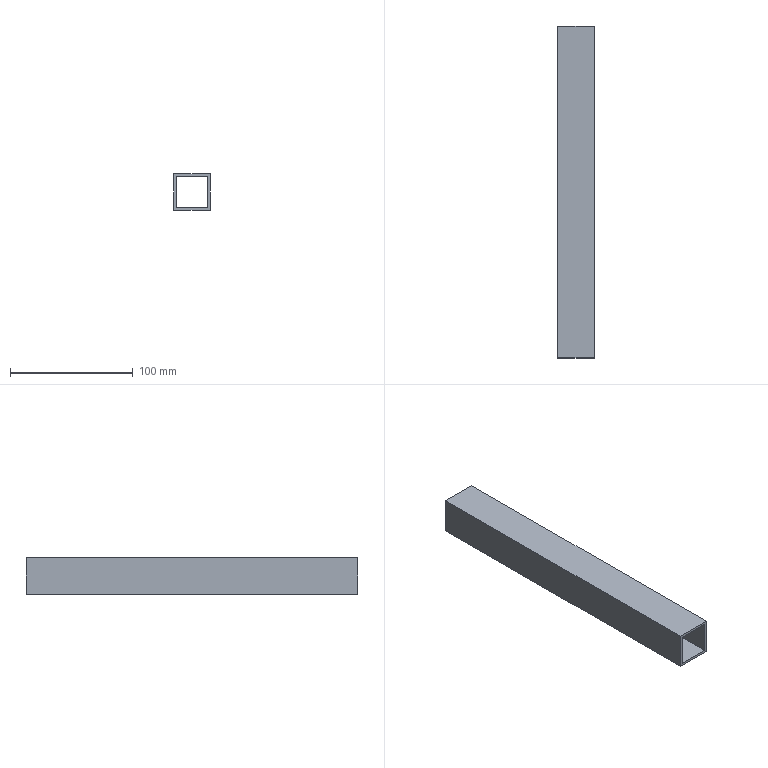Part | NX | features solid 2 | 1 solid | 10 faces | box 30 x 270 x 30 mm | volume 60480 mm3 | plane 10
STEP:
#1=CARTESIAN_POINT('',(230.,-350.,20.));
#2=VERTEX_POINT('',#1);
#3=CARTESIAN_POINT('',(200.,-350.,20.));
#4=VERTEX_POINT('',#3);
#5=CARTESIAN_POINT('',(230.,-350.,20.));
#6=DIRECTION('',(-1.,0.,0.));
#7=VECTOR('',#6,1000.);
#8=LINE('',#5,#7);
#9=EDGE_CURVE('',#2,#4,#8,.T.);
#10=ORIENTED_EDGE('',*,*,#9,.F.);
#11=CARTESIAN_POINT('',(230.,-620.,20.));
#12=VERTEX_POINT('',#11);
#13=CARTESIAN_POINT('',(230.,210.,20.));
#14=DIRECTION('',(0.,-1.,0.));
#15=VECTOR('',#14,1000.);
#16=LINE('',#13,#15);
#17=EDGE_CURVE('',#2,#12,#16,.T.);
#18=ORIENTED_EDGE('',*,*,#17,.T.);
#19=CARTESIAN_POINT('',(200.,-620.,20.));
#20=VERTEX_POINT('',#19);
#21=CARTESIAN_POINT('',(230.,-620.,20.));
#22=DIRECTION('',(1.,0.,0.));
#23=VECTOR('',#22,1000.);
#24=LINE('',#21,#23);
#25=EDGE_CURVE('',#20,#12,#24,.T.);
#26=ORIENTED_EDGE('',*,*,#25,.F.);
#27=CARTESIAN_POINT('',(200.,210.,20.));
#28=DIRECTION('',(0.,-1.,0.));
#29=VECTOR('',#28,1000.);
#30=LINE('',#27,#29);
#31=EDGE_CURVE('',#4,#20,#30,.T.);
#32=ORIENTED_EDGE('',*,*,#31,.F.);
#33=EDGE_LOOP('',(#10,#18,#26,#32));
#34=FACE_BOUND('',#33,.T.);
#35=CARTESIAN_POINT('',(230.,210.,20.));
#36=DIRECTION('',(0.,0.,-1.));
#37=DIRECTION('',(-1.,0.,0.));
#38=AXIS2_PLACEMENT_3D('',#35,#36,#37);
#39=PLANE('',#38);
#40=ADVANCED_FACE('',(#34),#39,.T.);
#41=CARTESIAN_POINT('',(230.,-350.,50.));
#42=VERTEX_POINT('',#41);
#43=CARTESIAN_POINT('',(230.,-620.,50.));
#44=VERTEX_POINT('',#43);
#45=CARTESIAN_POINT('',(230.,210.,50.));
#46=DIRECTION('',(0.,-1.,0.));
#47=VECTOR('',#46,1000.);
#48=LINE('',#45,#47);
#49=EDGE_CURVE('',#42,#44,#48,.T.);
#50=ORIENTED_EDGE('',*,*,#49,.F.);
#51=CARTESIAN_POINT('',(200.,-350.,50.));
#52=VERTEX_POINT('',#51);
#53=CARTESIAN_POINT('',(230.,-350.,50.));
#54=DIRECTION('',(-1.,0.,0.));
#55=VECTOR('',#54,1000.);
#56=LINE('',#53,#55);
#57=EDGE_CURVE('',#42,#52,#56,.T.);
#58=ORIENTED_EDGE('',*,*,#57,.T.);
#59=CARTESIAN_POINT('',(200.,-620.,50.));
#60=VERTEX_POINT('',#59);
#61=CARTESIAN_POINT('',(200.,210.,50.));
#62=DIRECTION('',(0.,-1.,0.));
#63=VECTOR('',#62,1000.);
#64=LINE('',#61,#63);
#65=EDGE_CURVE('',#52,#60,#64,.T.);
#66=ORIENTED_EDGE('',*,*,#65,.T.);
#67=CARTESIAN_POINT('',(230.,-620.,50.));
#68=DIRECTION('',(1.,0.,0.));
#69=VECTOR('',#68,1000.);
#70=LINE('',#67,#69);
#71=EDGE_CURVE('',#60,#44,#70,.T.);
#72=ORIENTED_EDGE('',*,*,#71,.T.);
#73=EDGE_LOOP('',(#50,#58,#66,#72));
#74=FACE_BOUND('',#73,.T.);
#75=CARTESIAN_POINT('',(230.,210.,50.));
#76=DIRECTION('',(0.,0.,-1.));
#77=DIRECTION('',(-1.,0.,0.));
#78=AXIS2_PLACEMENT_3D('',#75,#76,#77);
#79=PLANE('',#78);
#80=ADVANCED_FACE('',(#74),#79,.F.);
#81=ORIENTED_EDGE('',*,*,#65,.F.);
#82=CARTESIAN_POINT('',(200.,-350.,50.));
#83=DIRECTION('',(0.,0.,-1.));
#84=VECTOR('',#83,1000.);
#85=LINE('',#82,#84);
#86=EDGE_CURVE('',#52,#4,#85,.T.);
#87=ORIENTED_EDGE('',*,*,#86,.T.);
#88=ORIENTED_EDGE('',*,*,#31,.T.);
#89=CARTESIAN_POINT('',(200.,-620.,50.));
#90=DIRECTION('',(0.,0.,-1.));
#91=VECTOR('',#90,1000.);
#92=LINE('',#89,#91);
#93=EDGE_CURVE('',#60,#20,#92,.T.);
#94=ORIENTED_EDGE('',*,*,#93,.F.);
#95=EDGE_LOOP('',(#81,#87,#88,#94));
#96=FACE_BOUND('',#95,.T.);
#97=CARTESIAN_POINT('',(200.,210.,50.));
#98=DIRECTION('',(1.,0.,0.));
#99=DIRECTION('',(0.,0.,-1.));
#100=AXIS2_PLACEMENT_3D('',#97,#98,#99);
#101=PLANE('',#100);
#102=ADVANCED_FACE('',(#96),#101,.F.);
#103=CARTESIAN_POINT('',(230.,-350.,50.));
#104=DIRECTION('',(0.,0.,-1.));
#105=VECTOR('',#104,1000.);
#106=LINE('',#103,#105);
#107=EDGE_CURVE('',#42,#2,#106,.T.);
#108=ORIENTED_EDGE('',*,*,#107,.F.);
#109=ORIENTED_EDGE('',*,*,#49,.T.);
#110=CARTESIAN_POINT('',(230.,-620.,50.));
#111=DIRECTION('',(0.,0.,-1.));
#112=VECTOR('',#111,1000.);
#113=LINE('',#110,#112);
#114=EDGE_CURVE('',#44,#12,#113,.T.);
#115=ORIENTED_EDGE('',*,*,#114,.T.);
#116=ORIENTED_EDGE('',*,*,#17,.F.);
#117=EDGE_LOOP('',(#108,#109,#115,#116));
#118=FACE_BOUND('',#117,.T.);
#119=CARTESIAN_POINT('',(230.,210.,50.));
#120=DIRECTION('',(1.,0.,0.));
#121=DIRECTION('',(0.,0.,-1.));
#122=AXIS2_PLACEMENT_3D('',#119,#120,#121);
#123=PLANE('',#122);
#124=ADVANCED_FACE('',(#118),#123,.T.);
#125=ORIENTED_EDGE('',*,*,#25,.T.);
#126=ORIENTED_EDGE('',*,*,#114,.F.);
#127=ORIENTED_EDGE('',*,*,#71,.F.);
#128=ORIENTED_EDGE('',*,*,#93,.T.);
#129=EDGE_LOOP('',(#125,#126,#127,#128));
#130=FACE_BOUND('',#129,.T.);
#131=CARTESIAN_POINT('',(202.,-620.,22.));
#132=VERTEX_POINT('',#131);
#133=CARTESIAN_POINT('',(228.,-620.,22.));
#134=VERTEX_POINT('',#133);
#135=CARTESIAN_POINT('',(230.,-620.,22.));
#136=DIRECTION('',(1.,0.,0.));
#137=VECTOR('',#136,1000.);
#138=LINE('',#135,#137);
#139=EDGE_CURVE('',#132,#134,#138,.T.);
#140=ORIENTED_EDGE('',*,*,#139,.F.);
#141=CARTESIAN_POINT('',(202.,-620.,48.));
#142=VERTEX_POINT('',#141);
#143=CARTESIAN_POINT('',(202.,-620.,50.));
#144=DIRECTION('',(0.,0.,-1.));
#145=VECTOR('',#144,1000.);
#146=LINE('',#143,#145);
#147=EDGE_CURVE('',#142,#132,#146,.T.);
#148=ORIENTED_EDGE('',*,*,#147,.F.);
#149=CARTESIAN_POINT('',(228.,-620.,48.));
#150=VERTEX_POINT('',#149);
#151=CARTESIAN_POINT('',(230.,-620.,48.));
#152=DIRECTION('',(1.,0.,0.));
#153=VECTOR('',#152,1000.);
#154=LINE('',#151,#153);
#155=EDGE_CURVE('',#142,#150,#154,.T.);
#156=ORIENTED_EDGE('',*,*,#155,.T.);
#157=CARTESIAN_POINT('',(228.,-620.,50.));
#158=DIRECTION('',(0.,0.,-1.));
#159=VECTOR('',#158,1000.);
#160=LINE('',#157,#159);
#161=EDGE_CURVE('',#150,#134,#160,.T.);
#162=ORIENTED_EDGE('',*,*,#161,.T.);
#163=EDGE_LOOP('',(#140,#148,#156,#162));
#164=FACE_BOUND('',#163,.T.);
#165=CARTESIAN_POINT('',(200.,-620.,50.));
#166=DIRECTION('',(0.,1.,0.));
#167=DIRECTION('',(0.,0.,1.));
#168=AXIS2_PLACEMENT_3D('',#165,#166,#167);
#169=PLANE('',#168);
#170=ADVANCED_FACE('',(#130,#164),#169,.F.);
#171=CARTESIAN_POINT('',(228.,-350.,22.));
#172=VERTEX_POINT('',#171);
#173=CARTESIAN_POINT('',(228.,210.,22.));
#174=DIRECTION('',(0.,-1.,0.));
#175=VECTOR('',#174,1000.);
#176=LINE('',#173,#175);
#177=EDGE_CURVE('',#172,#134,#176,.T.);
#178=ORIENTED_EDGE('',*,*,#177,.F.);
#179=CARTESIAN_POINT('',(202.,-350.,22.));
#180=VERTEX_POINT('',#179);
#181=CARTESIAN_POINT('',(230.,-350.,22.));
#182=DIRECTION('',(-1.,0.,0.));
#183=VECTOR('',#182,1000.);
#184=LINE('',#181,#183);
#185=EDGE_CURVE('',#172,#180,#184,.T.);
#186=ORIENTED_EDGE('',*,*,#185,.T.);
#187=CARTESIAN_POINT('',(202.,210.,22.));
#188=DIRECTION('',(0.,-1.,0.));
#189=VECTOR('',#188,1000.);
#190=LINE('',#187,#189);
#191=EDGE_CURVE('',#180,#132,#190,.T.);
#192=ORIENTED_EDGE('',*,*,#191,.T.);
#193=ORIENTED_EDGE('',*,*,#139,.T.);
#194=EDGE_LOOP('',(#178,#186,#192,#193));
#195=FACE_BOUND('',#194,.T.);
#196=CARTESIAN_POINT('',(230.,210.,22.));
#197=DIRECTION('',(0.,0.,-1.));
#198=DIRECTION('',(-1.,0.,0.));
#199=AXIS2_PLACEMENT_3D('',#196,#197,#198);
#200=PLANE('',#199);
#201=ADVANCED_FACE('',(#195),#200,.F.);
#202=CARTESIAN_POINT('',(228.,-350.,48.));
#203=VERTEX_POINT('',#202);
#204=CARTESIAN_POINT('',(202.,-350.,48.));
#205=VERTEX_POINT('',#204);
#206=CARTESIAN_POINT('',(230.,-350.,48.));
#207=DIRECTION('',(-1.,0.,0.));
#208=VECTOR('',#207,1000.);
#209=LINE('',#206,#208);
#210=EDGE_CURVE('',#203,#205,#209,.T.);
#211=ORIENTED_EDGE('',*,*,#210,.F.);
#212=CARTESIAN_POINT('',(228.,210.,48.));
#213=DIRECTION('',(0.,-1.,0.));
#214=VECTOR('',#213,1000.);
#215=LINE('',#212,#214);
#216=EDGE_CURVE('',#203,#150,#215,.T.);
#217=ORIENTED_EDGE('',*,*,#216,.T.);
#218=ORIENTED_EDGE('',*,*,#155,.F.);
#219=CARTESIAN_POINT('',(202.,210.,48.));
#220=DIRECTION('',(0.,-1.,0.));
#221=VECTOR('',#220,1000.);
#222=LINE('',#219,#221);
#223=EDGE_CURVE('',#205,#142,#222,.T.);
#224=ORIENTED_EDGE('',*,*,#223,.F.);
#225=EDGE_LOOP('',(#211,#217,#218,#224));
#226=FACE_BOUND('',#225,.T.);
#227=CARTESIAN_POINT('',(230.,210.,48.));
#228=DIRECTION('',(0.,0.,-1.));
#229=DIRECTION('',(-1.,0.,0.));
#230=AXIS2_PLACEMENT_3D('',#227,#228,#229);
#231=PLANE('',#230);
#232=ADVANCED_FACE('',(#226),#231,.T.);
#233=CARTESIAN_POINT('',(202.,-350.,50.));
#234=DIRECTION('',(0.,0.,-1.));
#235=VECTOR('',#234,1000.);
#236=LINE('',#233,#235);
#237=EDGE_CURVE('',#205,#180,#236,.T.);
#238=ORIENTED_EDGE('',*,*,#237,.F.);
#239=ORIENTED_EDGE('',*,*,#223,.T.);
#240=ORIENTED_EDGE('',*,*,#147,.T.);
#241=ORIENTED_EDGE('',*,*,#191,.F.);
#242=EDGE_LOOP('',(#238,#239,#240,#241));
#243=FACE_BOUND('',#242,.T.);
#244=CARTESIAN_POINT('',(202.,210.,50.));
#245=DIRECTION('',(1.,0.,0.));
#246=DIRECTION('',(0.,0.,-1.));
#247=AXIS2_PLACEMENT_3D('',#244,#245,#246);
#248=PLANE('',#247);
#249=ADVANCED_FACE('',(#243),#248,.T.);
#250=ORIENTED_EDGE('',*,*,#216,.F.);
#251=CARTESIAN_POINT('',(228.,-350.,50.));
#252=DIRECTION('',(0.,0.,-1.));
#253=VECTOR('',#252,1000.);
#254=LINE('',#251,#253);
#255=EDGE_CURVE('',#203,#172,#254,.T.);
#256=ORIENTED_EDGE('',*,*,#255,.T.);
#257=ORIENTED_EDGE('',*,*,#177,.T.);
#258=ORIENTED_EDGE('',*,*,#161,.F.);
#259=EDGE_LOOP('',(#250,#256,#257,#258));
#260=FACE_BOUND('',#259,.T.);
#261=CARTESIAN_POINT('',(228.,210.,50.));
#262=DIRECTION('',(1.,0.,0.));
#263=DIRECTION('',(0.,0.,-1.));
#264=AXIS2_PLACEMENT_3D('',#261,#262,#263);
#265=PLANE('',#264);
#266=ADVANCED_FACE('',(#260),#265,.F.);
#267=ORIENTED_EDGE('',*,*,#210,.T.);
#268=ORIENTED_EDGE('',*,*,#237,.T.);
#269=ORIENTED_EDGE('',*,*,#185,.F.);
#270=ORIENTED_EDGE('',*,*,#255,.F.);
#271=EDGE_LOOP('',(#267,#268,#269,#270));
#272=FACE_BOUND('',#271,.T.);
#273=ORIENTED_EDGE('',*,*,#107,.T.);
#274=ORIENTED_EDGE('',*,*,#9,.T.);
#275=ORIENTED_EDGE('',*,*,#86,.F.);
#276=ORIENTED_EDGE('',*,*,#57,.F.);
#277=EDGE_LOOP('',(#273,#274,#275,#276));
#278=FACE_BOUND('',#277,.T.);
#279=CARTESIAN_POINT('',(200.,-350.,50.));
#280=DIRECTION('',(0.,-1.,0.));
#281=DIRECTION('',(0.,0.,-1.));
#282=AXIS2_PLACEMENT_3D('',#279,#280,#281);
#283=PLANE('',#282);
#284=ADVANCED_FACE('',(#272,#278),#283,.F.);
#285=CLOSED_SHELL('',(#40,#80,#102,#124,#170,#201,#232,#249,#266,#284));
#286=MANIFOLD_SOLID_BREP('',#285);
#287=(LENGTH_UNIT()NAMED_UNIT(*)SI_UNIT(.MILLI.,.METRE.));
#288=UNCERTAINTY_MEASURE_WITH_UNIT(LENGTH_MEASURE(0.00001),#287,'','');
#289=(NAMED_UNIT(*)PLANE_ANGLE_UNIT()SI_UNIT($,.RADIAN.));
#290=(NAMED_UNIT(*)SI_UNIT($,.STERADIAN.)SOLID_ANGLE_UNIT());
#291=(GEOMETRIC_REPRESENTATION_CONTEXT(3)GLOBAL_UNCERTAINTY_ASSIGNED_CONTEXT((#288))GLOBAL_UNIT_ASSIGNED_CONTEXT((#287,#289,#290))REPRESENTATION_CONTEXT('',''));
#292=ADVANCED_BREP_SHAPE_REPRESENTATION('',(#286),#291);